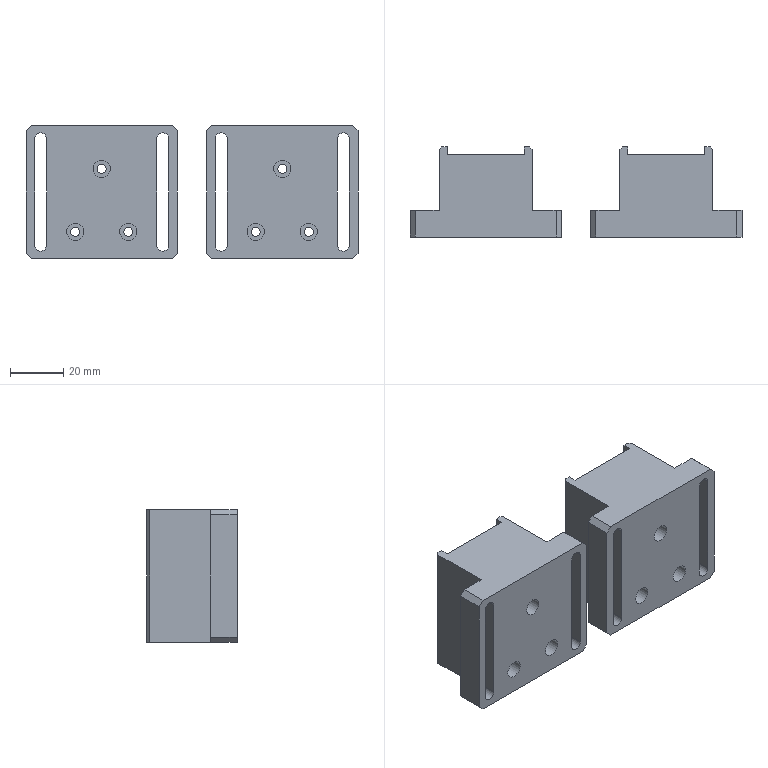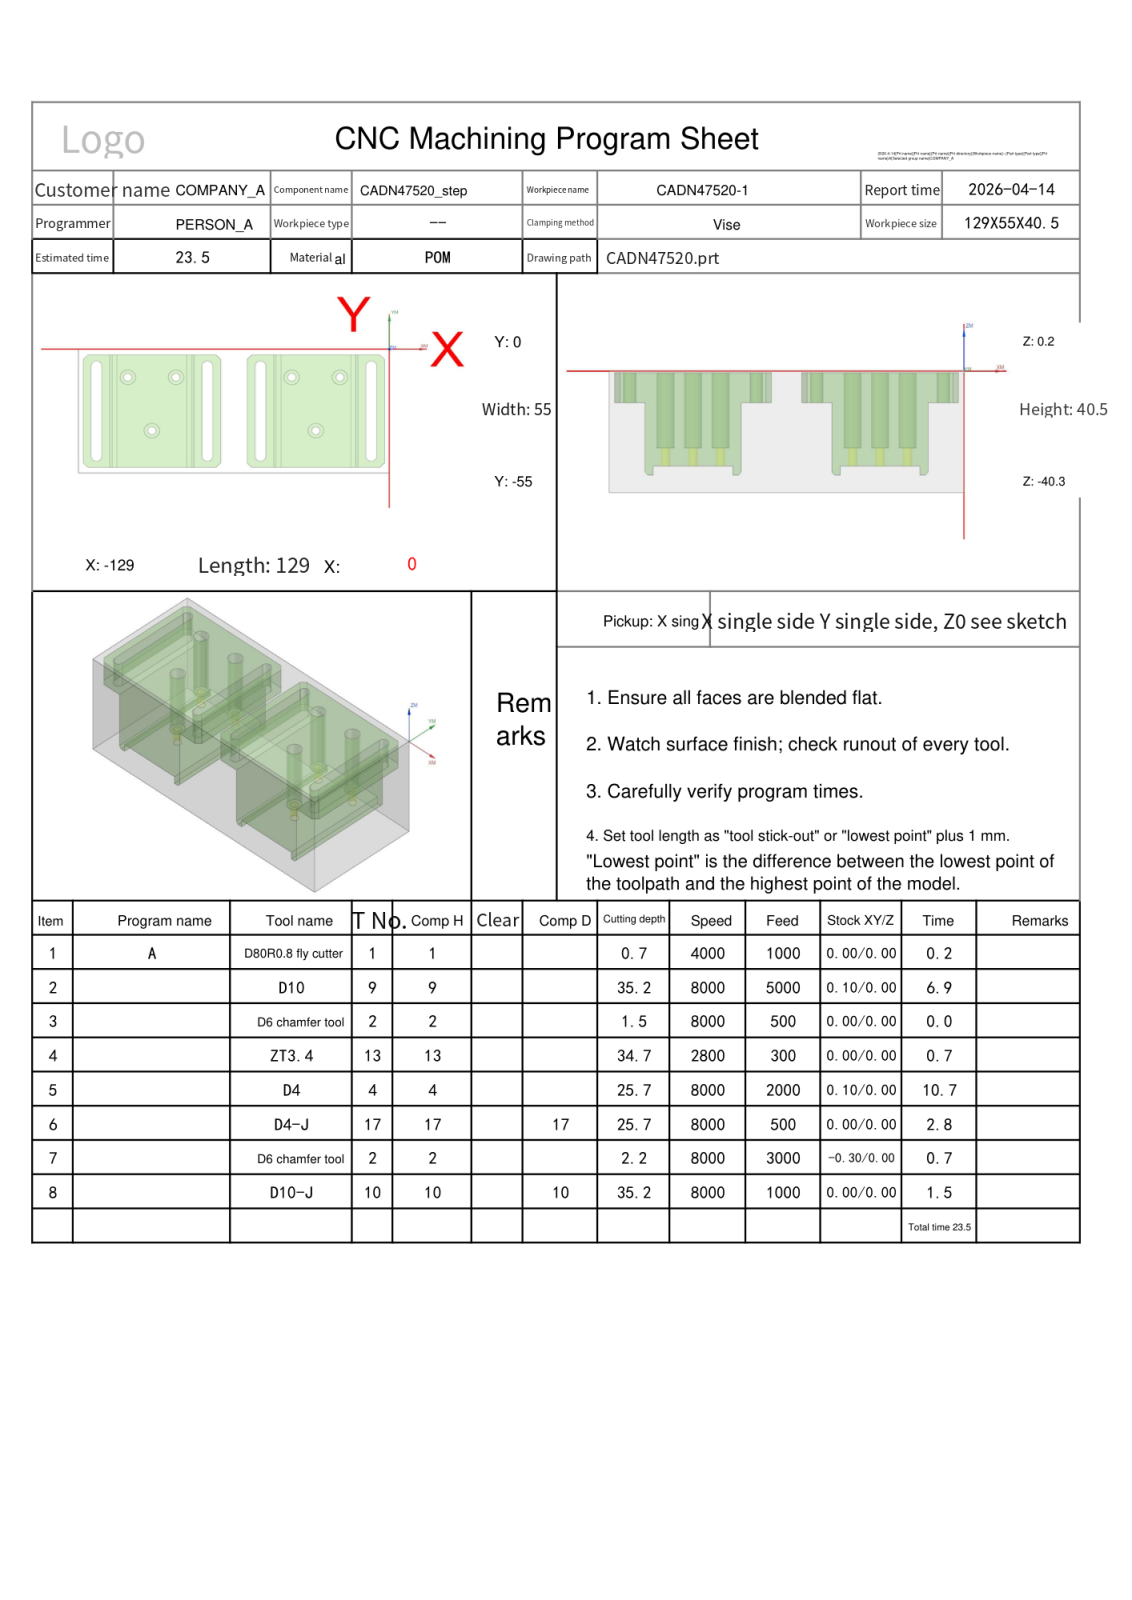NC program | NX | posted by the shop | part box 125 x 34 x 50 mm
Lines 1 to 33 of 5259:
%
O0001
(Machine time: 22.99 MIN)
(===Total Tool:7===)
(T1=D80R0.8 fly cutter D=80.  R=0.8  D-  H01 Z=-0.5  )
(T9=D10     D=10.  R=0.   D-  H09 Z=-35.  )
(T2=D6 chamfer tool   D=6.   R=0.   D-  H02 Z=-2.   )
(T13=ZT3.4  D=3.4  DR_a=118 D-  H13 Z=-34.52)
(T4=D4      D=4.   R=0.   D-  H04 Z=-25.5 )
(T17=D4-J   D=4.   R=0.   D17 H17 Z=-25.5 )
(T10=D10-J  D=10.  R=0.   D10 H10 Z=-35.  )
G80 G90 G17 G49 G40
G91 G28 Z0
M01
N1 T01 M06
(D80R0.8 fly cutter  D=80. R=0.8 H=01 ce=0.00 di=0.00)
G00 G90 G54 X-172. Y-27.5 M03 S4000
G43 H01 Z19.5
M08
Z1.5
G01 Z-.5 F1000.
X-167.
X38.
X43.
Z1.5
G00 Z19.5
G91 G28 Z0.0
M05
M09
G91 G28 Z0.0
M01